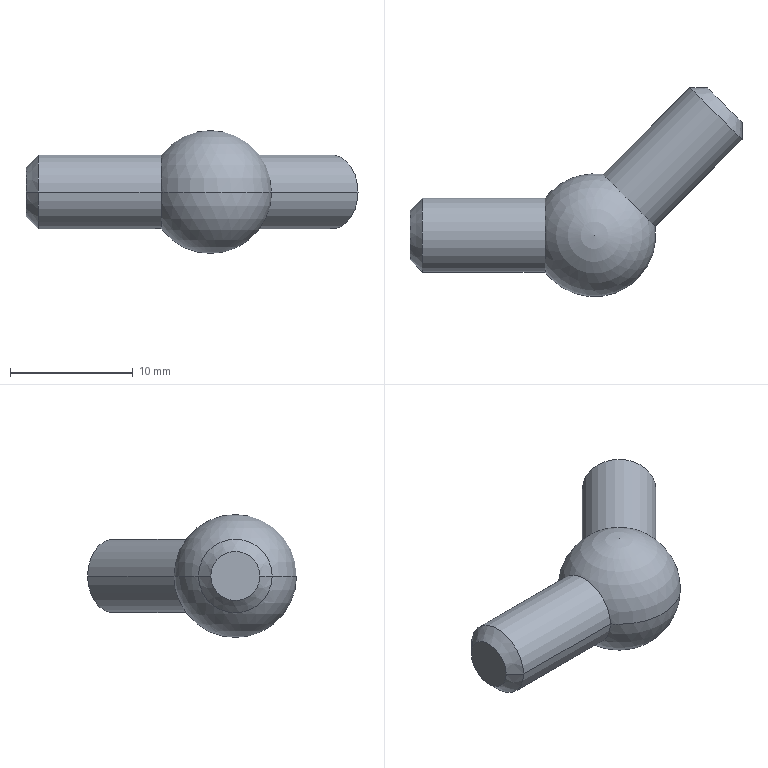Part | STEP file | [B-M6F] | 1 solid | 12 faces | box 27.021 x 17.021 x 10 mm | volume 1100 mm3 | cone 4 | cylinder 4 | sphere 2 | plane 2 | commonest cylinder face diameters 6 x4
STEP:
#1=CARTESIAN_POINT('',(0.,0.,0.));
#2=DIRECTION('',(0.,0.,1.));
#3=DIRECTION('',(1.,0.,0.));
#4=AXIS2_PLACEMENT_3D('',#1,#2,#3);
#5=CARTESIAN_POINT('',(174.099,-132.886,5.));
#6=VERTEX_POINT('',#5);
#7=CARTESIAN_POINT('',(171.271,-130.057,5.));
#8=VERTEX_POINT('',#7);
#9=CARTESIAN_POINT('',(172.685,-131.472,5.));
#10=DIRECTION('',(0.7071,0.7071,0.));
#11=DIRECTION('',(0.7071,-0.7071,0.));
#12=AXIS2_PLACEMENT_3D('',#9,#10,#11);
#13=CIRCLE('',#12,2.);
#14=CARTESIAN_POINT('',(171.978,-132.179,5.));
#15=DIRECTION('',(-0.7071,-0.7071,0.));
#16=DIRECTION('',(-0.7071,0.7071,0.));
#17=AXIS2_PLACEMENT_3D('',#14,#15,#16);
#18=CONICAL_SURFACE('',#17,3.,0.7854);
#19=CARTESIAN_POINT('',(3.142,-1.));
#20=DIRECTION('',(-1.,0.));
#21=VECTOR('',#20,1.);
#22=LINE('',#19,#21);
#23=(GEOMETRIC_REPRESENTATION_CONTEXT(2)PARAMETRIC_REPRESENTATION_CONTEXT()REPRESENTATION_CONTEXT('',''));
#24=DEFINITIONAL_REPRESENTATION('',(#22),#23);
#25=PCURVE('',#18,#24);
#26=CARTESIAN_POINT('',(172.685,-131.472,5.));
#27=DIRECTION('',(0.7071,0.7071,0.));
#28=DIRECTION('',(0.7071,-0.7071,0.));
#29=AXIS2_PLACEMENT_3D('',#26,#27,#28);
#30=PLANE('',#29);
#31=CARTESIAN_POINT('',(0.,0.));
#32=DIRECTION('',(1.,0.));
#33=AXIS2_PLACEMENT_2D('',#31,#32);
#34=CIRCLE('',#33,2.);
#35=(GEOMETRIC_REPRESENTATION_CONTEXT(2)PARAMETRIC_REPRESENTATION_CONTEXT()REPRESENTATION_CONTEXT('',''));
#36=DEFINITIONAL_REPRESENTATION('',(#34),#35);
#37=PCURVE('',#30,#36);
#38=SURFACE_CURVE('',#13,(#25,#37),.PCURVE_S1.);
#39=EDGE_CURVE('',#6,#8,#38,.T.);
#40=ORIENTED_EDGE('',*,*,#39,.F.);
#41=CARTESIAN_POINT('',(174.099,-134.3,5.));
#42=VERTEX_POINT('',#41);
#43=CARTESIAN_POINT('',(174.099,-134.3,5.));
#44=DIRECTION('',(0.,-1.,0.));
#45=VECTOR('',#44,1.);
#46=LINE('',#43,#45);
#47=CARTESIAN_POINT('',(3.142,0.));
#48=DIRECTION('',(0.,1.));
#49=VECTOR('',#48,1.);
#50=LINE('',#47,#49);
#51=(GEOMETRIC_REPRESENTATION_CONTEXT(2)PARAMETRIC_REPRESENTATION_CONTEXT()REPRESENTATION_CONTEXT('',''));
#52=DEFINITIONAL_REPRESENTATION('',(#50),#51);
#53=PCURVE('',#18,#52);
#54=CARTESIAN_POINT('',(171.978,-132.179,5.));
#55=DIRECTION('',(-0.7071,-0.7071,0.));
#56=DIRECTION('',(-0.7071,0.7071,0.));
#57=AXIS2_PLACEMENT_3D('',#54,#55,#56);
#58=CONICAL_SURFACE('',#57,3.,0.7854);
#59=CARTESIAN_POINT('',(3.142,0.));
#60=DIRECTION('',(0.,1.));
#61=VECTOR('',#60,1.);
#62=LINE('',#59,#61);
#63=(GEOMETRIC_REPRESENTATION_CONTEXT(2)PARAMETRIC_REPRESENTATION_CONTEXT()REPRESENTATION_CONTEXT('',''));
#64=DEFINITIONAL_REPRESENTATION('',(#62),#63);
#65=PCURVE('',#58,#64);
#66=SURFACE_CURVE('',#46,(#53,#65),.PCURVE_S1.);
#67=EDGE_CURVE('',#6,#42,#66,.T.);
#68=ORIENTED_EDGE('',*,*,#67,.T.);
#69=CARTESIAN_POINT('',(169.856,-130.057,5.));
#70=VERTEX_POINT('',#69);
#71=CARTESIAN_POINT('',(171.978,-132.179,5.));
#72=DIRECTION('',(-0.7071,-0.7071,0.));
#73=DIRECTION('',(0.7071,-0.7071,0.));
#74=AXIS2_PLACEMENT_3D('',#71,#72,#73);
#75=CIRCLE('',#74,3.);
#76=CARTESIAN_POINT('',(-3.142,0.));
#77=DIRECTION('',(1.,0.));
#78=VECTOR('',#77,1.);
#79=LINE('',#76,#78);
#80=(GEOMETRIC_REPRESENTATION_CONTEXT(2)PARAMETRIC_REPRESENTATION_CONTEXT()REPRESENTATION_CONTEXT('',''));
#81=DEFINITIONAL_REPRESENTATION('',(#79),#80);
#82=PCURVE('',#18,#81);
#83=CARTESIAN_POINT('',(172.685,-131.472,5.));
#84=DIRECTION('',(-0.7071,-0.7071,0.));
#85=DIRECTION('',(-0.7071,0.7071,0.));
#86=AXIS2_PLACEMENT_3D('',#83,#84,#85);
#87=CYLINDRICAL_SURFACE('',#86,3.);
#88=CARTESIAN_POINT('',(-3.142,1.));
#89=DIRECTION('',(1.,0.));
#90=VECTOR('',#89,1.);
#91=LINE('',#88,#90);
#92=(GEOMETRIC_REPRESENTATION_CONTEXT(2)PARAMETRIC_REPRESENTATION_CONTEXT()REPRESENTATION_CONTEXT('',''));
#93=DEFINITIONAL_REPRESENTATION('',(#91),#92);
#94=PCURVE('',#87,#93);
#95=SURFACE_CURVE('',#75,(#82,#94),.PCURVE_S1.);
#96=EDGE_CURVE('',#70,#42,#95,.T.);
#97=ORIENTED_EDGE('',*,*,#96,.F.);
#98=CARTESIAN_POINT('',(169.856,-130.057,5.));
#99=DIRECTION('',(-1.,0.,0.));
#100=VECTOR('',#99,1.);
#101=LINE('',#98,#100);
#102=CARTESIAN_POINT('',(0.,0.));
#103=DIRECTION('',(0.,1.));
#104=VECTOR('',#103,1.);
#105=LINE('',#102,#104);
#106=(GEOMETRIC_REPRESENTATION_CONTEXT(2)PARAMETRIC_REPRESENTATION_CONTEXT()REPRESENTATION_CONTEXT('',''));
#107=DEFINITIONAL_REPRESENTATION('',(#105),#106);
#108=PCURVE('',#18,#107);
#109=CARTESIAN_POINT('',(6.283,0.));
#110=DIRECTION('',(0.,1.));
#111=VECTOR('',#110,1.);
#112=LINE('',#109,#111);
#113=(GEOMETRIC_REPRESENTATION_CONTEXT(2)PARAMETRIC_REPRESENTATION_CONTEXT()REPRESENTATION_CONTEXT('',''));
#114=DEFINITIONAL_REPRESENTATION('',(#112),#113);
#115=PCURVE('',#58,#114);
#116=SURFACE_CURVE('',#101,(#108,#115),.PCURVE_S1.);
#117=EDGE_CURVE('',#8,#70,#116,.T.);
#118=ORIENTED_EDGE('',*,*,#117,.F.);
#119=EDGE_LOOP('',(#40,#68,#97,#118));
#120=FACE_BOUND('',#119,.T.);
#121=ADVANCED_FACE('',(#120),#18,.T.);
#122=CARTESIAN_POINT('',(147.078,-140.078,5.));
#123=VERTEX_POINT('',#122);
#124=CARTESIAN_POINT('',(147.078,-144.078,5.));
#125=VERTEX_POINT('',#124);
#126=CARTESIAN_POINT('',(147.078,-142.078,5.));
#127=DIRECTION('',(-1.,0.,0.));
#128=DIRECTION('',(0.,1.,0.));
#129=AXIS2_PLACEMENT_3D('',#126,#127,#128);
#130=CIRCLE('',#129,2.);
#131=CARTESIAN_POINT('',(148.078,-142.078,5.));
#132=DIRECTION('',(1.,0.,0.));
#133=DIRECTION('',(0.,-1.,0.));
#134=AXIS2_PLACEMENT_3D('',#131,#132,#133);
#135=CONICAL_SURFACE('',#134,3.,0.7854);
#136=CARTESIAN_POINT('',(3.142,-1.));
#137=DIRECTION('',(-1.,0.));
#138=VECTOR('',#137,1.);
#139=LINE('',#136,#138);
#140=(GEOMETRIC_REPRESENTATION_CONTEXT(2)PARAMETRIC_REPRESENTATION_CONTEXT()REPRESENTATION_CONTEXT('',''));
#141=DEFINITIONAL_REPRESENTATION('',(#139),#140);
#142=PCURVE('',#135,#141);
#143=CARTESIAN_POINT('',(147.078,-142.078,5.));
#144=DIRECTION('',(-1.,0.,0.));
#145=DIRECTION('',(0.,1.,0.));
#146=AXIS2_PLACEMENT_3D('',#143,#144,#145);
#147=PLANE('',#146);
#148=CARTESIAN_POINT('',(0.,0.));
#149=DIRECTION('',(1.,0.));
#150=AXIS2_PLACEMENT_2D('',#148,#149);
#151=CIRCLE('',#150,2.);
#152=(GEOMETRIC_REPRESENTATION_CONTEXT(2)PARAMETRIC_REPRESENTATION_CONTEXT()REPRESENTATION_CONTEXT('',''));
#153=DEFINITIONAL_REPRESENTATION('',(#151),#152);
#154=PCURVE('',#147,#153);
#155=SURFACE_CURVE('',#130,(#142,#154),.PCURVE_S1.);
#156=EDGE_CURVE('',#123,#125,#155,.T.);
#157=ORIENTED_EDGE('',*,*,#156,.F.);
#158=CARTESIAN_POINT('',(148.078,-139.078,5.));
#159=VERTEX_POINT('',#158);
#160=CARTESIAN_POINT('',(148.078,-139.078,5.));
#161=DIRECTION('',(0.7071,0.7071,0.));
#162=VECTOR('',#161,1.);
#163=LINE('',#160,#162);
#164=CARTESIAN_POINT('',(3.142,0.));
#165=DIRECTION('',(0.,1.));
#166=VECTOR('',#165,1.);
#167=LINE('',#164,#166);
#168=(GEOMETRIC_REPRESENTATION_CONTEXT(2)PARAMETRIC_REPRESENTATION_CONTEXT()REPRESENTATION_CONTEXT('',''));
#169=DEFINITIONAL_REPRESENTATION('',(#167),#168);
#170=PCURVE('',#135,#169);
#171=CARTESIAN_POINT('',(148.078,-142.078,5.));
#172=DIRECTION('',(1.,0.,0.));
#173=DIRECTION('',(0.,-1.,0.));
#174=AXIS2_PLACEMENT_3D('',#171,#172,#173);
#175=CONICAL_SURFACE('',#174,3.,0.7854);
#176=CARTESIAN_POINT('',(3.142,0.));
#177=DIRECTION('',(0.,1.));
#178=VECTOR('',#177,1.);
#179=LINE('',#176,#178);
#180=(GEOMETRIC_REPRESENTATION_CONTEXT(2)PARAMETRIC_REPRESENTATION_CONTEXT()REPRESENTATION_CONTEXT('',''));
#181=DEFINITIONAL_REPRESENTATION('',(#179),#180);
#182=PCURVE('',#175,#181);
#183=SURFACE_CURVE('',#163,(#170,#182),.PCURVE_S1.);
#184=EDGE_CURVE('',#123,#159,#183,.T.);
#185=ORIENTED_EDGE('',*,*,#184,.T.);
#186=CARTESIAN_POINT('',(148.078,-145.078,5.));
#187=VERTEX_POINT('',#186);
#188=CARTESIAN_POINT('',(148.078,-142.078,5.));
#189=DIRECTION('',(1.,0.,0.));
#190=DIRECTION('',(0.,1.,0.));
#191=AXIS2_PLACEMENT_3D('',#188,#189,#190);
#192=CIRCLE('',#191,3.);
#193=CARTESIAN_POINT('',(-3.142,0.));
#194=DIRECTION('',(1.,0.));
#195=VECTOR('',#194,1.);
#196=LINE('',#193,#195);
#197=(GEOMETRIC_REPRESENTATION_CONTEXT(2)PARAMETRIC_REPRESENTATION_CONTEXT()REPRESENTATION_CONTEXT('',''));
#198=DEFINITIONAL_REPRESENTATION('',(#196),#197);
#199=PCURVE('',#135,#198);
#200=CARTESIAN_POINT('',(147.078,-142.078,5.));
#201=DIRECTION('',(1.,0.,0.));
#202=DIRECTION('',(0.,-1.,0.));
#203=AXIS2_PLACEMENT_3D('',#200,#201,#202);
#204=CYLINDRICAL_SURFACE('',#203,3.);
#205=CARTESIAN_POINT('',(-3.142,1.));
#206=DIRECTION('',(1.,0.));
#207=VECTOR('',#206,1.);
#208=LINE('',#205,#207);
#209=(GEOMETRIC_REPRESENTATION_CONTEXT(2)PARAMETRIC_REPRESENTATION_CONTEXT()REPRESENTATION_CONTEXT('',''));
#210=DEFINITIONAL_REPRESENTATION('',(#208),#209);
#211=PCURVE('',#204,#210);
#212=SURFACE_CURVE('',#192,(#199,#211),.PCURVE_S1.);
#213=EDGE_CURVE('',#187,#159,#212,.T.);
#214=ORIENTED_EDGE('',*,*,#213,.F.);
#215=CARTESIAN_POINT('',(148.078,-145.078,5.));
#216=DIRECTION('',(0.7071,-0.7071,0.));
#217=VECTOR('',#216,1.);
#218=LINE('',#215,#217);
#219=CARTESIAN_POINT('',(0.,0.));
#220=DIRECTION('',(0.,1.));
#221=VECTOR('',#220,1.);
#222=LINE('',#219,#221);
#223=(GEOMETRIC_REPRESENTATION_CONTEXT(2)PARAMETRIC_REPRESENTATION_CONTEXT()REPRESENTATION_CONTEXT('',''));
#224=DEFINITIONAL_REPRESENTATION('',(#222),#223);
#225=PCURVE('',#135,#224);
#226=CARTESIAN_POINT('',(6.283,0.));
#227=DIRECTION('',(0.,1.));
#228=VECTOR('',#227,1.);
#229=LINE('',#226,#228);
#230=(GEOMETRIC_REPRESENTATION_CONTEXT(2)PARAMETRIC_REPRESENTATION_CONTEXT()REPRESENTATION_CONTEXT('',''));
#231=DEFINITIONAL_REPRESENTATION('',(#229),#230);
#232=PCURVE('',#175,#231);
#233=SURFACE_CURVE('',#218,(#225,#232),.PCURVE_S1.);
#234=EDGE_CURVE('',#125,#187,#233,.T.);
#235=ORIENTED_EDGE('',*,*,#234,.F.);
#236=EDGE_LOOP('',(#157,#185,#214,#235));
#237=FACE_BOUND('',#236,.T.);
#238=ADVANCED_FACE('',(#237),#135,.T.);
#239=ORIENTED_EDGE('',*,*,#96,.T.);
#240=CARTESIAN_POINT('',(167.028,-141.371,5.));
#241=VERTEX_POINT('',#240);
#242=CARTESIAN_POINT('',(174.806,-133.593,5.));
#243=DIRECTION('',(-0.7071,-0.7071,0.));
#244=VECTOR('',#243,1.);
#245=LINE('',#242,#244);
#246=CARTESIAN_POINT('',(3.142,0.));
#247=DIRECTION('',(0.,1.));
#248=VECTOR('',#247,1.);
#249=LINE('',#246,#248);
#250=(GEOMETRIC_REPRESENTATION_CONTEXT(2)PARAMETRIC_REPRESENTATION_CONTEXT()REPRESENTATION_CONTEXT('',''));
#251=DEFINITIONAL_REPRESENTATION('',(#249),#250);
#252=PCURVE('',#87,#251);
#253=CARTESIAN_POINT('',(172.685,-131.472,5.));
#254=DIRECTION('',(-0.7071,-0.7071,0.));
#255=DIRECTION('',(-0.7071,0.7071,0.));
#256=AXIS2_PLACEMENT_3D('',#253,#254,#255);
#257=CYLINDRICAL_SURFACE('',#256,3.);
#258=CARTESIAN_POINT('',(3.142,0.));
#259=DIRECTION('',(0.,1.));
#260=VECTOR('',#259,1.);
#261=LINE('',#258,#260);
#262=(GEOMETRIC_REPRESENTATION_CONTEXT(2)PARAMETRIC_REPRESENTATION_CONTEXT()REPRESENTATION_CONTEXT('',''));
#263=DEFINITIONAL_REPRESENTATION('',(#261),#262);
#264=PCURVE('',#257,#263);
#265=SURFACE_CURVE('',#245,(#252,#264),.PCURVE_S1.);
#266=EDGE_CURVE('',#42,#241,#265,.T.);
#267=ORIENTED_EDGE('',*,*,#266,.T.);
#268=CARTESIAN_POINT('',(162.785,-137.128,5.));
#269=VERTEX_POINT('',#268);
#270=CARTESIAN_POINT('',(164.907,-139.25,5.));
#271=DIRECTION('',(0.7071,0.7071,0.));
#272=DIRECTION('',(-0.7071,0.7071,0.));
#273=AXIS2_PLACEMENT_3D('',#270,#271,#272);
#274=CIRCLE('',#273,3.);
#275=CARTESIAN_POINT('',(6.283,11.));
#276=DIRECTION('',(-1.,0.));
#277=VECTOR('',#276,1.);
#278=LINE('',#275,#277);
#279=(GEOMETRIC_REPRESENTATION_CONTEXT(2)PARAMETRIC_REPRESENTATION_CONTEXT()REPRESENTATION_CONTEXT('',''));
#280=DEFINITIONAL_REPRESENTATION('',(#278),#279);
#281=PCURVE('',#87,#280);
#282=CARTESIAN_POINT('',(162.078,-142.078,5.));
#283=DIRECTION('',(0.,0.,-1.));
#284=DIRECTION('',(-0.7071,0.7071,0.));
#285=AXIS2_PLACEMENT_3D('',#282,#283,#284);
#286=SPHERICAL_SURFACE('',#285,5.);
#287=CARTESIAN_POINT('',(2.214,0.));
#288=CARTESIAN_POINT('',(2.214,0.02855));
#289=CARTESIAN_POINT('',(2.211,0.08568));
#290=CARTESIAN_POINT('',(2.196,0.1702));
#291=CARTESIAN_POINT('',(2.171,0.2525));
#292=CARTESIAN_POINT('',(2.136,0.3312));
#293=CARTESIAN_POINT('',(2.088,0.4049));
#294=CARTESIAN_POINT('',(2.029,0.472));
#295=CARTESIAN_POINT('',(1.958,0.5308));
#296=CARTESIAN_POINT('',(1.875,0.5793));
#297=CARTESIAN_POINT('',(1.78,0.6158));
#298=CARTESIAN_POINT('',(1.678,0.6384));
#299=CARTESIAN_POINT('',(1.571,0.6461));
#300=CARTESIAN_POINT('',(1.464,0.6384));
#301=CARTESIAN_POINT('',(1.361,0.6158));
#302=CARTESIAN_POINT('',(1.267,0.5793));
#303=CARTESIAN_POINT('',(1.184,0.5308));
#304=CARTESIAN_POINT('',(1.112,0.472));
#305=CARTESIAN_POINT('',(1.053,0.4049));
#306=CARTESIAN_POINT('',(1.006,0.3312));
#307=CARTESIAN_POINT('',(0.9703,0.2525));
#308=CARTESIAN_POINT('',(0.9453,0.1702));
#309=CARTESIAN_POINT('',(0.9305,0.08568));
#310=CARTESIAN_POINT('',(0.9273,0.02855));
#311=CARTESIAN_POINT('',(0.9273,0.));
#312=B_SPLINE_CURVE_WITH_KNOTS('',3,(#287,#288,#289,#290,#291,#292,#293,#294,#295,#296,#297,#298,#299,#300,#301,#302,#303,#304,#305,#306,#307,#308,#309,#310,#311),.UNSPECIFIED.,.F.,.F.,(4,1,1,1,1,1,1,1,1,1,1,1,1,1,1,1,1,1,1,1,1,1,4),(3.142,3.284,3.427,3.57,3.713,3.856,3.998,4.141,4.284,4.427,4.57,4.712,4.855,4.998,5.141,5.284,5.426,5.569,5.712,5.855,5.998,6.14,6.283),.QUASI_UNIFORM_KNOTS.);
#313=(GEOMETRIC_REPRESENTATION_CONTEXT(2)PARAMETRIC_REPRESENTATION_CONTEXT()REPRESENTATION_CONTEXT('',''));
#314=DEFINITIONAL_REPRESENTATION('',(#312),#313);
#315=PCURVE('',#286,#314);
#316=SURFACE_CURVE('',#274,(#281,#315),.PCURVE_S1.);
#317=EDGE_CURVE('',#241,#269,#316,.T.);
#318=ORIENTED_EDGE('',*,*,#317,.T.);
#319=CARTESIAN_POINT('',(170.563,-129.35,5.));
#320=DIRECTION('',(-0.7071,-0.7071,0.));
#321=VECTOR('',#320,1.);
#322=LINE('',#319,#321);
#323=CARTESIAN_POINT('',(0.,0.));
#324=DIRECTION('',(0.,1.));
#325=VECTOR('',#324,1.);
#326=LINE('',#323,#325);
#327=(GEOMETRIC_REPRESENTATION_CONTEXT(2)PARAMETRIC_REPRESENTATION_CONTEXT()REPRESENTATION_CONTEXT('',''));
#328=DEFINITIONAL_REPRESENTATION('',(#326),#327);
#329=PCURVE('',#87,#328);
#330=CARTESIAN_POINT('',(6.283,0.));
#331=DIRECTION('',(0.,1.));
#332=VECTOR('',#331,1.);
#333=LINE('',#330,#332);
#334=(GEOMETRIC_REPRESENTATION_CONTEXT(2)PARAMETRIC_REPRESENTATION_CONTEXT()REPRESENTATION_CONTEXT('',''));
#335=DEFINITIONAL_REPRESENTATION('',(#333),#334);
#336=PCURVE('',#257,#335);
#337=SURFACE_CURVE('',#322,(#329,#336),.PCURVE_S1.);
#338=EDGE_CURVE('',#70,#269,#337,.T.);
#339=ORIENTED_EDGE('',*,*,#338,.F.);
#340=EDGE_LOOP('',(#239,#267,#318,#339));
#341=FACE_BOUND('',#340,.T.);
#342=ADVANCED_FACE('',(#341),#87,.T.);
#343=ORIENTED_EDGE('',*,*,#317,.F.);
#344=CARTESIAN_POINT('',(158.543,-145.614,5.));
#345=VERTEX_POINT('',#344);
#346=CARTESIAN_POINT('',(162.078,-142.078,5.));
#347=DIRECTION('',(0.,0.,-1.));
#348=DIRECTION('',(-1.,0.,0.));
#349=AXIS2_PLACEMENT_3D('',#346,#347,#348);
#350=CIRCLE('',#349,5.);
#351=CARTESIAN_POINT('',(-0.7854,0.));
#352=DIRECTION('',(1.,0.));
#353=VECTOR('',#352,1.);
#354=LINE('',#351,#353);
#355=(GEOMETRIC_REPRESENTATION_CONTEXT(2)PARAMETRIC_REPRESENTATION_CONTEXT()REPRESENTATION_CONTEXT('',''));
#356=DEFINITIONAL_REPRESENTATION('',(#354),#355);
#357=PCURVE('',#286,#356);
#358=CARTESIAN_POINT('',(162.078,-142.078,5.));
#359=DIRECTION('',(0.,0.,-1.));
#360=DIRECTION('',(-0.7071,0.7071,0.));
#361=AXIS2_PLACEMENT_3D('',#358,#359,#360);
#362=SPHERICAL_SURFACE('',#361,5.);
#363=CARTESIAN_POINT('',(-0.7854,0.));
#364=DIRECTION('',(1.,0.));
#365=VECTOR('',#364,1.);
#366=LINE('',#363,#365);
#367=(GEOMETRIC_REPRESENTATION_CONTEXT(2)PARAMETRIC_REPRESENTATION_CONTEXT()REPRESENTATION_CONTEXT('',''));
#368=DEFINITIONAL_REPRESENTATION('',(#366),#367);
#369=PCURVE('',#362,#368);
#370=SURFACE_CURVE('',#350,(#357,#369),.PCURVE_S1.);
#371=EDGE_CURVE('',#241,#345,#370,.T.);
#372=ORIENTED_EDGE('',*,*,#371,.T.);
#373=CARTESIAN_POINT('',(158.078,-145.078,5.));
#374=VERTEX_POINT('',#373);
#375=CARTESIAN_POINT('',(162.078,-142.078,5.));
#376=DIRECTION('',(0.,0.,1.));
#377=DIRECTION('',(1.,0.,0.));
#378=AXIS2_PLACEMENT_3D('',#375,#376,#377);
#379=CIRCLE('',#378,5.);
#380=CARTESIAN_POINT('',(8.639,0.));
#381=DIRECTION('',(-1.,0.));
#382=VECTOR('',#381,1.);
#383=LINE('',#380,#382);
#384=(GEOMETRIC_REPRESENTATION_CONTEXT(2)PARAMETRIC_REPRESENTATION_CONTEXT()REPRESENTATION_CONTEXT('',''));
#385=DEFINITIONAL_REPRESENTATION('',(#383),#384);
#386=PCURVE('',#286,#385);
#387=CARTESIAN_POINT('',(8.639,0.));
#388=DIRECTION('',(-1.,0.));
#389=VECTOR('',#388,1.);
#390=LINE('',#387,#389);
#391=(GEOMETRIC_REPRESENTATION_CONTEXT(2)PARAMETRIC_REPRESENTATION_CONTEXT()REPRESENTATION_CONTEXT('',''));
#392=DEFINITIONAL_REPRESENTATION('',(#390),#391);
#393=PCURVE('',#362,#392);
#394=SURFACE_CURVE('',#379,(#386,#393),.PCURVE_S1.);
#395=EDGE_CURVE('',#374,#345,#394,.T.);
#396=ORIENTED_EDGE('',*,*,#395,.F.);
#397=CARTESIAN_POINT('',(158.078,-139.078,5.));
#398=VERTEX_POINT('',#397);
#399=CARTESIAN_POINT('',(158.078,-142.078,5.));
#400=DIRECTION('',(-1.,0.,0.));
#401=DIRECTION('',(0.,-1.,0.));
#402=AXIS2_PLACEMENT_3D('',#399,#400,#401);
#403=CIRCLE('',#402,3.);
#404=CARTESIAN_POINT('',(6.141,0.));
#405=CARTESIAN_POINT('',(6.141,0.02855));
#406=CARTESIAN_POINT('',(6.138,0.08568));
#407=CARTESIAN_POINT('',(6.123,0.1702));
#408=CARTESIAN_POINT('',(6.098,0.2525));
#409=CARTESIAN_POINT('',(6.063,0.3312));
#410=CARTESIAN_POINT('',(6.015,0.4049));
#411=CARTESIAN_POINT('',(5.956,0.472));
#412=CARTESIAN_POINT('',(5.885,0.5308));
#413=CARTESIAN_POINT('',(5.802,0.5793));
#414=CARTESIAN_POINT('',(5.707,0.6158));
#415=CARTESIAN_POINT('',(5.605,0.6384));
#416=CARTESIAN_POINT('',(5.498,0.6461));
#417=CARTESIAN_POINT('',(5.391,0.6384));
#418=CARTESIAN_POINT('',(5.288,0.6158));
#419=CARTESIAN_POINT('',(5.194,0.5793));
#420=CARTESIAN_POINT('',(5.111,0.5308));
#421=CARTESIAN_POINT('',(5.039,0.472));
#422=CARTESIAN_POINT('',(4.98,0.4049));
#423=CARTESIAN_POINT('',(4.933,0.3312));
#424=CARTESIAN_POINT('',(4.897,0.2525));
#425=CARTESIAN_POINT('',(4.872,0.1702));
#426=CARTESIAN_POINT('',(4.858,0.08568));
#427=CARTESIAN_POINT('',(4.854,0.02855));
#428=CARTESIAN_POINT('',(4.854,0.));
#429=B_SPLINE_CURVE_WITH_KNOTS('',3,(#404,#405,#406,#407,#408,#409,#410,#411,#412,#413,#414,#415,#416,#417,#418,#419,#420,#421,#422,#423,#424,#425,#426,#427,#428),.UNSPECIFIED.,.F.,.F.,(4,1,1,1,1,1,1,1,1,1,1,1,1,1,1,1,1,1,1,1,1,1,4),(3.142,3.284,3.427,3.57,3.713,3.856,3.998,4.141,4.284,4.427,4.57,4.712,4.855,4.998,5.141,5.284,5.426,5.569,5.712,5.855,5.998,6.14,6.283),.QUASI_UNIFORM_KNOTS.);
#430=(GEOMETRIC_REPRESENTATION_CONTEXT(2)PARAMETRIC_REPRESENTATION_CONTEXT()REPRESENTATION_CONTEXT('',''));
#431=DEFINITIONAL_REPRESENTATION('',(#429),#430);
#432=PCURVE('',#286,#431);
#433=CARTESIAN_POINT('',(6.283,11.));
#434=DIRECTION('',(-1.,0.));
#435=VECTOR('',#434,1.);
#436=LINE('',#433,#435);
#437=(GEOMETRIC_REPRESENTATION_CONTEXT(2)PARAMETRIC_REPRESENTATION_CONTEXT()REPRESENTATION_CONTEXT('',''));
#438=DEFINITIONAL_REPRESENTATION('',(#436),#437);
#439=PCURVE('',#204,#438);
#440=SURFACE_CURVE('',#403,(#432,#439),.PCURVE_S1.);
#441=EDGE_CURVE('',#398,#374,#440,.T.);
#442=ORIENTED_EDGE('',*,*,#441,.F.);
#443=CARTESIAN_POINT('',(158.543,-138.543,5.));
#444=VERTEX_POINT('',#443);
#445=CARTESIAN_POINT('',(162.078,-142.078,5.));
#446=DIRECTION('',(0.,0.,1.));
#447=DIRECTION('',(1.,0.,0.));
#448=AXIS2_PLACEMENT_3D('',#445,#446,#447);
#449=CIRCLE('',#448,5.);
#450=CARTESIAN_POINT('',(7.21,0.));
#451=CARTESIAN_POINT('',(7.194,0.));
#452=CARTESIAN_POINT('',(7.162,0.));
#453=CARTESIAN_POINT('',(7.113,0.));
#454=CARTESIAN_POINT('',(7.065,0.));
#455=CARTESIAN_POINT('',(7.016,0.));
#456=CARTESIAN_POINT('',(6.967,0.));
#457=CARTESIAN_POINT('',(6.919,0.));
#458=CARTESIAN_POINT('',(6.87,0.));
#459=CARTESIAN_POINT('',(6.822,0.));
#460=CARTESIAN_POINT('',(6.773,0.));
#461=CARTESIAN_POINT('',(6.724,0.));
#462=CARTESIAN_POINT('',(6.676,0.));
#463=CARTESIAN_POINT('',(6.627,0.));
#464=CARTESIAN_POINT('',(6.579,0.));
#465=CARTESIAN_POINT('',(6.53,0.));
#466=CARTESIAN_POINT('',(6.481,0.));
#467=CARTESIAN_POINT('',(6.433,0.));
#468=CARTESIAN_POINT('',(6.384,0.));
#469=CARTESIAN_POINT('',(6.336,0.));
#470=CARTESIAN_POINT('',(6.287,0.));
#471=CARTESIAN_POINT('',(6.238,0.));
#472=CARTESIAN_POINT('',(6.19,0.));
#473=CARTESIAN_POINT('',(6.157,0.));
#474=CARTESIAN_POINT('',(6.141,0.));
#475=B_SPLINE_CURVE_WITH_KNOTS('',3,(#450,#451,#452,#453,#454,#455,#456,#457,#458,#459,#460,#461,#462,#463,#464,#465,#466,#467,#468,#469,#470,#471,#472,#473,#474),.UNSPECIFIED.,.F.,.F.,(4,1,1,1,1,1,1,1,1,1,1,1,1,1,1,1,1,1,1,1,1,1,4),(1.429,1.477,1.526,1.575,1.623,1.672,1.72,1.769,1.818,1.866,1.915,1.963,2.012,2.061,2.109,2.158,2.206,2.255,2.304,2.352,2.401,2.449,2.498),.QUASI_UNIFORM_KNOTS.);
#476=(GEOMETRIC_REPRESENTATION_CONTEXT(2)PARAMETRIC_REPRESENTATION_CONTEXT()REPRESENTATION_CONTEXT('',''));
#477=DEFINITIONAL_REPRESENTATION('',(#475),#476);
#478=PCURVE('',#286,#477);
#479=CARTESIAN_POINT('',(6.283,0.));
#480=CARTESIAN_POINT('',(6.281,0.));
#481=CARTESIAN_POINT('',(6.277,0.));
#482=CARTESIAN_POINT('',(6.27,0.));
#483=CARTESIAN_POINT('',(6.264,0.));
#484=CARTESIAN_POINT('',(6.257,0.));
#485=CARTESIAN_POINT('',(6.251,0.));
#486=CARTESIAN_POINT('',(6.244,0.));
#487=CARTESIAN_POINT('',(6.238,0.));
#488=CARTESIAN_POINT('',(6.232,0.));
#489=CARTESIAN_POINT('',(6.225,0.));
#490=CARTESIAN_POINT('',(6.219,0.));
#491=CARTESIAN_POINT('',(6.212,0.));
#492=CARTESIAN_POINT('',(6.206,0.));
#493=CARTESIAN_POINT('',(6.199,0.));
#494=CARTESIAN_POINT('',(6.193,0.));
#495=CARTESIAN_POINT('',(6.186,0.));
#496=CARTESIAN_POINT('',(6.18,0.));
#497=CARTESIAN_POINT('',(6.174,0.));
#498=CARTESIAN_POINT('',(6.167,0.));
#499=CARTESIAN_POINT('',(6.161,0.));
#500=CARTESIAN_POINT('',(6.154,0.));
#501=CARTESIAN_POINT('',(6.148,0.));
#502=CARTESIAN_POINT('',(6.143,0.));
#503=CARTESIAN_POINT('',(6.141,0.));
#504=B_SPLINE_CURVE_WITH_KNOTS('',3,(#479,#480,#481,#482,#483,#484,#485,#486,#487,#488,#489,#490,#491,#492,#493,#494,#495,#496,#497,#498,#499,#500,#501,#502,#503),.UNSPECIFIED.,.F.,.F.,(4,1,1,1,1,1,1,1,1,1,1,1,1,1,1,1,1,1,1,1,1,1,4),(2.356,2.363,2.369,2.376,2.382,2.388,2.395,2.401,2.408,2.414,2.421,2.427,2.434,2.44,2.446,2.453,2.459,2.466,2.472,2.479,2.485,2.492,2.498),.QUASI_UNIFORM_KNOTS.);
#505=(GEOMETRIC_REPRESENTATION_CONTEXT(2)PARAMETRIC_REPRESENTATION_CONTEXT()REPRESENTATION_CONTEXT('',''));
#506=DEFINITIONAL_REPRESENTATION('',(#504),#505);
#507=PCURVE('',#362,#506);
#508=SURFACE_CURVE('',#449,(#478,#507),.PCURVE_S1.);
#509=EDGE_CURVE('',#444,#398,#508,.T.);
#510=ORIENTED_EDGE('',*,*,#509,.F.);
#511=CARTESIAN_POINT('',(162.078,-142.078,0.));
#512=VERTEX_POINT('',#511);
#513=CARTESIAN_POINT('',(158.543,-138.543,5.));
#514=CARTESIAN_POINT('',(158.543,-138.543,3.691));
#515=CARTESIAN_POINT('',(158.833,-138.833,2.382));
#516=CARTESIAN_POINT('',(159.415,-139.415,1.234));
#517=CARTESIAN_POINT('',(160.227,-140.227,0.4111));
#518=CARTESIAN_POINT('',(161.153,-141.153,0.));
#519=CARTESIAN_POINT('',(162.078,-142.078,0.));
#520=B_SPLINE_CURVE_WITH_KNOTS('',6,(#513,#514,#515,#516,#517,#518,#519),.UNSPECIFIED.,.F.,.F.,(7,7),(0.,1.571),.PIECEWISE_BEZIER_KNOTS.);
#521=CARTESIAN_POINT('',(6.283,0.));
#522=DIRECTION('',(0.,1.));
#523=VECTOR('',#522,1.);
#524=LINE('',#521,#523);
#525=(GEOMETRIC_REPRESENTATION_CONTEXT(2)PARAMETRIC_REPRESENTATION_CONTEXT()REPRESENTATION_CONTEXT('',''));
#526=DEFINITIONAL_REPRESENTATION('',(#524),#525);
#527=PCURVE('',#286,#526);
#528=CARTESIAN_POINT('',(0.,0.));
#529=DIRECTION('',(0.,1.));
#530=VECTOR('',#529,1.);
#531=LINE('',#528,#530);
#532=(GEOMETRIC_REPRESENTATION_CONTEXT(2)PARAMETRIC_REPRESENTATION_CONTEXT()REPRESENTATION_CONTEXT('',''));
#533=DEFINITIONAL_REPRESENTATION('',(#531),#532);
#534=PCURVE('',#286,#533);
#535=SEAM_CURVE('',#520,(#527,#534),.PCURVE_S1.);
#536=EDGE_CURVE('',#444,#512,#535,.T.);
#537=ORIENTED_EDGE('',*,*,#536,.T.);
#538=ORIENTED_EDGE('',*,*,#536,.F.);
#539=CARTESIAN_POINT('',(162.078,-142.078,5.));
#540=DIRECTION('',(0.,0.,1.));
#541=DIRECTION('',(1.,0.,0.));
#542=AXIS2_PLACEMENT_3D('',#539,#540,#541);
#543=CIRCLE('',#542,5.);
#544=CARTESIAN_POINT('',(0.9273,0.));
#545=CARTESIAN_POINT('',(0.9111,0.));
#546=CARTESIAN_POINT('',(0.8787,0.));
#547=CARTESIAN_POINT('',(0.8301,0.));
#548=CARTESIAN_POINT('',(0.7815,0.));
#549=CARTESIAN_POINT('',(0.7329,0.));
#550=CARTESIAN_POINT('',(0.6843,0.));
#551=CARTESIAN_POINT('',(0.6357,0.));
#552=CARTESIAN_POINT('',(0.5871,0.));
#553=CARTESIAN_POINT('',(0.5385,0.));
#554=CARTESIAN_POINT('',(0.4899,0.));
#555=CARTESIAN_POINT('',(0.4413,0.));
#556=CARTESIAN_POINT('',(0.3927,0.));
#557=CARTESIAN_POINT('',(0.3441,0.));
#558=CARTESIAN_POINT('',(0.2955,0.));
#559=CARTESIAN_POINT('',(0.2469,0.));
#560=CARTESIAN_POINT('',(0.1983,0.));
#561=CARTESIAN_POINT('',(0.1497,0.));
#562=CARTESIAN_POINT('',(0.1011,0.));
#563=CARTESIAN_POINT('',(0.0525,0.));
#564=CARTESIAN_POINT('',(0.003902,0.));
#565=CARTESIAN_POINT('',(-0.0447,0.));
#566=CARTESIAN_POINT('',(-0.0933,0.));
#567=CARTESIAN_POINT('',(-0.1257,0.));
#568=CARTESIAN_POINT('',(-0.1419,0.));
#569=B_SPLINE_CURVE_WITH_KNOTS('',3,(#544,#545,#546,#547,#548,#549,#550,#551,#552,#553,#554,#555,#556,#557,#558,#559,#560,#561,#562,#563,#564,#565,#566,#567,#568),.UNSPECIFIED.,.F.,.F.,(4,1,1,1,1,1,1,1,1,1,1,1,1,1,1,1,1,1,1,1,1,1,4),(1.429,1.477,1.526,1.575,1.623,1.672,1.72,1.769,1.818,1.866,1.915,1.963,2.012,2.061,2.109,2.158,2.206,2.255,2.304,2.352,2.401,2.449,2.498),.QUASI_UNIFORM_KNOTS.);
#570=(GEOMETRIC_REPRESENTATION_CONTEXT(2)PARAMETRIC_REPRESENTATION_CONTEXT()REPRESENTATION_CONTEXT('',''));
#571=DEFINITIONAL_REPRESENTATION('',(#569),#570);
#572=PCURVE('',#286,#571);
#573=CARTESIAN_POINT('',(2.356,0.));
#574=DIRECTION('',(-1.,0.));
#575=VECTOR('',#574,1.);
#576=LINE('',#573,#575);
#577=(GEOMETRIC_REPRESENTATION_CONTEXT(2)PARAMETRIC_REPRESENTATION_CONTEXT()REPRESENTATION_CONTEXT('',''));
#578=DEFINITIONAL_REPRESENTATION('',(#576),#577);
#579=PCURVE('',#362,#578);
#580=SURFACE_CURVE('',#543,(#572,#579),.PCURVE_S1.);
#581=EDGE_CURVE('',#269,#444,#580,.T.);
#582=ORIENTED_EDGE('',*,*,#581,.F.);
#583=EDGE_LOOP('',(#343,#372,#396,#442,#510,#537,#538,#582));
#584=FACE_BOUND('',#583,.T.);
#585=ADVANCED_FACE('',(#584),#286,.T.);
#586=ORIENTED_EDGE('',*,*,#213,.T.);
#587=CARTESIAN_POINT('',(147.078,-139.078,5.));
#588=DIRECTION('',(1.,0.,0.));
#589=VECTOR('',#588,1.);
#590=LINE('',#587,#589);
#591=CARTESIAN_POINT('',(3.142,0.));
#592=DIRECTION('',(0.,1.));
#593=VECTOR('',#592,1.);
#594=LINE('',#591,#593);
#595=(GEOMETRIC_REPRESENTATION_CONTEXT(2)PARAMETRIC_REPRESENTATION_CONTEXT()REPRESENTATION_CONTEXT('',''));
#596=DEFINITIONAL_REPRESENTATION('',(#594),#595);
#597=PCURVE('',#204,#596);
#598=CARTESIAN_POINT('',(147.078,-142.078,5.));
#599=DIRECTION('',(1.,0.,0.));
#600=DIRECTION('',(0.,-1.,0.));
#601=AXIS2_PLACEMENT_3D('',#598,#599,#600);
#602=CYLINDRICAL_SURFACE('',#601,3.);
#603=CARTESIAN_POINT('',(3.142,0.));
#604=DIRECTION('',(0.,1.));
#605=VECTOR('',#604,1.);
#606=LINE('',#603,#605);
#607=(GEOMETRIC_REPRESENTATION_CONTEXT(2)PARAMETRIC_REPRESENTATION_CONTEXT()REPRESENTATION_CONTEXT('',''));
#608=DEFINITIONAL_REPRESENTATION('',(#606),#607);
#609=PCURVE('',#602,#608);
#610=SURFACE_CURVE('',#590,(#597,#609),.PCURVE_S1.);
#611=EDGE_CURVE('',#159,#398,#610,.T.);
#612=ORIENTED_EDGE('',*,*,#611,.T.);
#613=ORIENTED_EDGE('',*,*,#441,.T.);
#614=CARTESIAN_POINT('',(147.078,-145.078,5.));
#615=DIRECTION('',(1.,0.,0.));
#616=VECTOR('',#615,1.);
#617=LINE('',#614,#616);
#618=CARTESIAN_POINT('',(0.,0.));
#619=DIRECTION('',(0.,1.));
#620=VECTOR('',#619,1.);
#621=LINE('',#618,#620);
#622=(GEOMETRIC_REPRESENTATION_CONTEXT(2)PARAMETRIC_REPRESENTATION_CONTEXT()REPRESENTATION_CONTEXT('',''));
#623=DEFINITIONAL_REPRESENTATION('',(#621),#622);
#624=PCURVE('',#204,#623);
#625=CARTESIAN_POINT('',(6.283,0.));
#626=DIRECTION('',(0.,1.));
#627=VECTOR('',#626,1.);
#628=LINE('',#625,#627);
#629=(GEOMETRIC_REPRESENTATION_CONTEXT(2)PARAMETRIC_REPRESENTATION_CONTEXT()REPRESENTATION_CONTEXT('',''));
#630=DEFINITIONAL_REPRESENTATION('',(#628),#629);
#631=PCURVE('',#602,#630);
#632=SURFACE_CURVE('',#617,(#624,#631),.PCURVE_S1.);
#633=EDGE_CURVE('',#187,#374,#632,.T.);
#634=ORIENTED_EDGE('',*,*,#633,.F.);
#635=EDGE_LOOP('',(#586,#612,#613,#634));
#636=FACE_BOUND('',#635,.T.);
#637=ADVANCED_FACE('',(#636),#204,.T.);
#638=CARTESIAN_POINT('',(147.078,-142.078,5.));
#639=DIRECTION('',(-1.,0.,0.));
#640=DIRECTION('',(0.,1.,0.));
#641=AXIS2_PLACEMENT_3D('',#638,#639,#640);
#642=CIRCLE('',#641,2.);
#643=CARTESIAN_POINT('',(0.,0.));
#644=DIRECTION('',(1.,0.));
#645=AXIS2_PLACEMENT_2D('',#643,#644);
#646=CIRCLE('',#645,2.);
#647=(GEOMETRIC_REPRESENTATION_CONTEXT(2)PARAMETRIC_REPRESENTATION_CONTEXT()REPRESENTATION_CONTEXT('',''));
#648=DEFINITIONAL_REPRESENTATION('',(#646),#647);
#649=PCURVE('',#147,#648);
#650=CARTESIAN_POINT('',(9.425,-1.));
#651=DIRECTION('',(-1.,0.));
#652=VECTOR('',#651,1.);
#653=LINE('',#650,#652);
#654=(GEOMETRIC_REPRESENTATION_CONTEXT(2)PARAMETRIC_REPRESENTATION_CONTEXT()REPRESENTATION_CONTEXT('',''));
#655=DEFINITIONAL_REPRESENTATION('',(#653),#654);
#656=PCURVE('',#175,#655);
#657=SURFACE_CURVE('',#642,(#649,#656),.PCURVE_S1.);
#658=EDGE_CURVE('',#125,#123,#657,.T.);
#659=ORIENTED_EDGE('',*,*,#658,.T.);
#660=ORIENTED_EDGE('',*,*,#156,.T.);
#661=EDGE_LOOP('',(#659,#660));
#662=FACE_BOUND('',#661,.T.);
#663=ADVANCED_FACE('',(#662),#147,.T.);
#664=ORIENTED_EDGE('',*,*,#611,.F.);
#665=CARTESIAN_POINT('',(148.078,-142.078,5.));
#666=DIRECTION('',(1.,0.,0.));
#667=DIRECTION('',(0.,1.,0.));
#668=AXIS2_PLACEMENT_3D('',#665,#666,#667);
#669=CIRCLE('',#668,3.);
#670=CARTESIAN_POINT('',(3.142,1.));
#671=DIRECTION('',(1.,0.));
#672=VECTOR('',#671,1.);
#673=LINE('',#670,#672);
#674=(GEOMETRIC_REPRESENTATION_CONTEXT(2)PARAMETRIC_REPRESENTATION_CONTEXT()REPRESENTATION_CONTEXT('',''));
#675=DEFINITIONAL_REPRESENTATION('',(#673),#674);
#676=PCURVE('',#602,#675);
#677=CARTESIAN_POINT('',(3.142,0.));
#678=DIRECTION('',(1.,0.));
#679=VECTOR('',#678,1.);
#680=LINE('',#677,#679);
#681=(GEOMETRIC_REPRESENTATION_CONTEXT(2)PARAMETRIC_REPRESENTATION_CONTEXT()REPRESENTATION_CONTEXT('',''));
#682=DEFINITIONAL_REPRESENTATION('',(#680),#681);
#683=PCURVE('',#175,#682);
#684=SURFACE_CURVE('',#669,(#676,#683),.PCURVE_S1.);
#685=EDGE_CURVE('',#159,#187,#684,.T.);
#686=ORIENTED_EDGE('',*,*,#685,.T.);
#687=ORIENTED_EDGE('',*,*,#633,.T.);
#688=CARTESIAN_POINT('',(158.078,-142.078,5.));
#689=DIRECTION('',(-1.,0.,0.));
#690=DIRECTION('',(0.,-1.,0.));
#691=AXIS2_PLACEMENT_3D('',#688,#689,#690);
#692=CIRCLE('',#691,3.);
#693=CARTESIAN_POINT('',(6.283,11.));
#694=DIRECTION('',(-1.,0.));
#695=VECTOR('',#694,1.);
#696=LINE('',#693,#695);
#697=(GEOMETRIC_REPRESENTATION_CONTEXT(2)PARAMETRIC_REPRESENTATION_CONTEXT()REPRESENTATION_CONTEXT('',''));
#698=DEFINITIONAL_REPRESENTATION('',(#696),#697);
#699=PCURVE('',#602,#698);
#700=CARTESIAN_POINT('',(4.854,0.));
#701=CARTESIAN_POINT('',(4.854,-0.02855));
#702=CARTESIAN_POINT('',(4.858,-0.08568));
#703=CARTESIAN_POINT('',(4.872,-0.1702));
#704=CARTESIAN_POINT('',(4.897,-0.2525));
#705=CARTESIAN_POINT('',(4.933,-0.3312));
#706=CARTESIAN_POINT('',(4.98,-0.4049));
#707=CARTESIAN_POINT('',(5.039,-0.472));
#708=CARTESIAN_POINT('',(5.111,-0.5308));
#709=CARTESIAN_POINT('',(5.194,-0.5793));
#710=CARTESIAN_POINT('',(5.288,-0.6158));
#711=CARTESIAN_POINT('',(5.391,-0.6384));
#712=CARTESIAN_POINT('',(5.498,-0.6461));
#713=CARTESIAN_POINT('',(5.605,-0.6384));
#714=CARTESIAN_POINT('',(5.707,-0.6158));
#715=CARTESIAN_POINT('',(5.802,-0.5793));
#716=CARTESIAN_POINT('',(5.885,-0.5308));
#717=CARTESIAN_POINT('',(5.956,-0.472));
#718=CARTESIAN_POINT('',(6.015,-0.4049));
#719=CARTESIAN_POINT('',(6.063,-0.3312));
#720=CARTESIAN_POINT('',(6.098,-0.2525));
#721=CARTESIAN_POINT('',(6.123,-0.1702));
#722=CARTESIAN_POINT('',(6.138,-0.08568));
#723=CARTESIAN_POINT('',(6.141,-0.02855));
#724=CARTESIAN_POINT('',(6.141,0.));
#725=B_SPLINE_CURVE_WITH_KNOTS('',3,(#700,#701,#702,#703,#704,#705,#706,#707,#708,#709,#710,#711,#712,#713,#714,#715,#716,#717,#718,#719,#720,#721,#722,#723,#724),.UNSPECIFIED.,.F.,.F.,(4,1,1,1,1,1,1,1,1,1,1,1,1,1,1,1,1,1,1,1,1,1,4),(0.,0.1428,0.2856,0.4284,0.5712,0.714,0.8568,0.9996,1.142,1.285,1.428,1.571,1.714,1.856,1.999,2.142,2.285,2.428,2.57,2.713,2.856,2.999,3.142),.QUASI_UNIFORM_KNOTS.);
#726=(GEOMETRIC_REPRESENTATION_CONTEXT(2)PARAMETRIC_REPRESENTATION_CONTEXT()REPRESENTATION_CONTEXT('',''));
#727=DEFINITIONAL_REPRESENTATION('',(#725),#726);
#728=PCURVE('',#362,#727);
#729=SURFACE_CURVE('',#692,(#699,#728),.PCURVE_S1.);
#730=EDGE_CURVE('',#374,#398,#729,.T.);
#731=ORIENTED_EDGE('',*,*,#730,.T.);
#732=EDGE_LOOP('',(#664,#686,#687,#731));
#733=FACE_BOUND('',#732,.T.);
#734=ADVANCED_FACE('',(#733),#602,.T.);
#735=ORIENTED_EDGE('',*,*,#371,.F.);
#736=CARTESIAN_POINT('',(164.907,-139.25,5.));
#737=DIRECTION('',(0.7071,0.7071,0.));
#738=DIRECTION('',(-0.7071,0.7071,0.));
#739=AXIS2_PLACEMENT_3D('',#736,#737,#738);
#740=CIRCLE('',#739,3.);
#741=CARTESIAN_POINT('',(0.9273,0.));
#742=CARTESIAN_POINT('',(0.9273,-0.02855));
#743=CARTESIAN_POINT('',(0.9305,-0.08568));
#744=CARTESIAN_POINT('',(0.9453,-0.1702));
#745=CARTESIAN_POINT('',(0.9703,-0.2525));
#746=CARTESIAN_POINT('',(1.006,-0.3312));
#747=CARTESIAN_POINT('',(1.053,-0.4049));
#748=CARTESIAN_POINT('',(1.112,-0.472));
#749=CARTESIAN_POINT('',(1.184,-0.5308));
#750=CARTESIAN_POINT('',(1.267,-0.5793));
#751=CARTESIAN_POINT('',(1.361,-0.6158));
#752=CARTESIAN_POINT('',(1.464,-0.6384));
#753=CARTESIAN_POINT('',(1.571,-0.6461));
#754=CARTESIAN_POINT('',(1.678,-0.6384));
#755=CARTESIAN_POINT('',(1.78,-0.6158));
#756=CARTESIAN_POINT('',(1.875,-0.5793));
#757=CARTESIAN_POINT('',(1.958,-0.5308));
#758=CARTESIAN_POINT('',(2.029,-0.472));
#759=CARTESIAN_POINT('',(2.088,-0.4049));
#760=CARTESIAN_POINT('',(2.136,-0.3312));
#761=CARTESIAN_POINT('',(2.171,-0.2525));
#762=CARTESIAN_POINT('',(2.196,-0.1702));
#763=CARTESIAN_POINT('',(2.211,-0.08568));
#764=CARTESIAN_POINT('',(2.214,-0.02855));
#765=CARTESIAN_POINT('',(2.214,0.));
#766=B_SPLINE_CURVE_WITH_KNOTS('',3,(#741,#742,#743,#744,#745,#746,#747,#748,#749,#750,#751,#752,#753,#754,#755,#756,#757,#758,#759,#760,#761,#762,#763,#764,#765),.UNSPECIFIED.,.F.,.F.,(4,1,1,1,1,1,1,1,1,1,1,1,1,1,1,1,1,1,1,1,1,1,4),(0.,0.1428,0.2856,0.4284,0.5712,0.714,0.8568,0.9996,1.142,1.285,1.428,1.571,1.714,1.856,1.999,2.142,2.285,2.428,2.57,2.713,2.856,2.999,3.142),.QUASI_UNIFORM_KNOTS.);
#767=(GEOMETRIC_REPRESENTATION_CONTEXT(2)PARAMETRIC_REPRESENTATION_CONTEXT()REPRESENTATION_CONTEXT('',''));
#768=DEFINITIONAL_REPRESENTATION('',(#766),#767);
#769=PCURVE('',#362,#768);
#770=CARTESIAN_POINT('',(6.283,11.));
#771=DIRECTION('',(-1.,0.));
#772=VECTOR('',#771,1.);
#773=LINE('',#770,#772);
#774=(GEOMETRIC_REPRESENTATION_CONTEXT(2)PARAMETRIC_REPRESENTATION_CONTEXT()REPRESENTATION_CONTEXT('',''));
#775=DEFINITIONAL_REPRESENTATION('',(#773),#774);
#776=PCURVE('',#257,#775);
#777=SURFACE_CURVE('',#740,(#769,#776),.PCURVE_S1.);
#778=EDGE_CURVE('',#269,#241,#777,.T.);
#779=ORIENTED_EDGE('',*,*,#778,.F.);
#780=ORIENTED_EDGE('',*,*,#581,.T.);
#781=CARTESIAN_POINT('',(162.078,-142.078,10.));
#782=VERTEX_POINT('',#781);
#783=CARTESIAN_POINT('',(162.078,-142.078,10.));
#784=CARTESIAN_POINT('',(161.153,-141.153,10.));
#785=CARTESIAN_POINT('',(160.227,-140.227,9.589));
#786=CARTESIAN_POINT('',(159.415,-139.415,8.766));
#787=CARTESIAN_POINT('',(158.833,-138.833,7.618));
#788=CARTESIAN_POINT('',(158.543,-138.543,6.309));
#789=CARTESIAN_POINT('',(158.543,-138.543,5.));
#790=B_SPLINE_CURVE_WITH_KNOTS('',6,(#783,#784,#785,#786,#787,#788,#789),.UNSPECIFIED.,.F.,.F.,(7,7),(-1.571,0.),.PIECEWISE_BEZIER_KNOTS.);
#791=CARTESIAN_POINT('',(0.,0.));
#792=DIRECTION('',(0.,1.));
#793=VECTOR('',#792,1.);
#794=LINE('',#791,#793);
#795=(GEOMETRIC_REPRESENTATION_CONTEXT(2)PARAMETRIC_REPRESENTATION_CONTEXT()REPRESENTATION_CONTEXT('',''));
#796=DEFINITIONAL_REPRESENTATION('',(#794),#795);
#797=PCURVE('',#362,#796);
#798=CARTESIAN_POINT('',(6.283,0.));
#799=DIRECTION('',(0.,1.));
#800=VECTOR('',#799,1.);
#801=LINE('',#798,#800);
#802=(GEOMETRIC_REPRESENTATION_CONTEXT(2)PARAMETRIC_REPRESENTATION_CONTEXT()REPRESENTATION_CONTEXT('',''));
#803=DEFINITIONAL_REPRESENTATION('',(#801),#802);
#804=PCURVE('',#362,#803);
#805=SEAM_CURVE('',#790,(#797,#804),.PCURVE_S1.);
#806=EDGE_CURVE('',#782,#444,#805,.T.);
#807=ORIENTED_EDGE('',*,*,#806,.F.);
#808=ORIENTED_EDGE('',*,*,#806,.T.);
#809=ORIENTED_EDGE('',*,*,#509,.T.);
#810=ORIENTED_EDGE('',*,*,#730,.F.);
#811=ORIENTED_EDGE('',*,*,#395,.T.);
#812=EDGE_LOOP('',(#735,#779,#780,#807,#808,#809,#810,#811));
#813=FACE_BOUND('',#812,.T.);
#814=ADVANCED_FACE('',(#813),#362,.T.);
#815=CARTESIAN_POINT('',(172.685,-131.472,5.));
#816=DIRECTION('',(0.7071,0.7071,0.));
#817=DIRECTION('',(0.7071,-0.7071,0.));
#818=AXIS2_PLACEMENT_3D('',#815,#816,#817);
#819=CIRCLE('',#818,2.);
#820=CARTESIAN_POINT('',(0.,0.));
#821=DIRECTION('',(1.,0.));
#822=AXIS2_PLACEMENT_2D('',#820,#821);
#823=CIRCLE('',#822,2.);
#824=(GEOMETRIC_REPRESENTATION_CONTEXT(2)PARAMETRIC_REPRESENTATION_CONTEXT()REPRESENTATION_CONTEXT('',''));
#825=DEFINITIONAL_REPRESENTATION('',(#823),#824);
#826=PCURVE('',#30,#825);
#827=CARTESIAN_POINT('',(9.425,-1.));
#828=DIRECTION('',(-1.,0.));
#829=VECTOR('',#828,1.);
#830=LINE('',#827,#829);
#831=(GEOMETRIC_REPRESENTATION_CONTEXT(2)PARAMETRIC_REPRESENTATION_CONTEXT()REPRESENTATION_CONTEXT('',''));
#832=DEFINITIONAL_REPRESENTATION('',(#830),#831);
#833=PCURVE('',#58,#832);
#834=SURFACE_CURVE('',#819,(#826,#833),.PCURVE_S1.);
#835=EDGE_CURVE('',#8,#6,#834,.T.);
#836=ORIENTED_EDGE('',*,*,#835,.T.);
#837=ORIENTED_EDGE('',*,*,#39,.T.);
#838=EDGE_LOOP('',(#836,#837));
#839=FACE_BOUND('',#838,.T.);
#840=ADVANCED_FACE('',(#839),#30,.T.);
#841=ORIENTED_EDGE('',*,*,#266,.F.);
#842=CARTESIAN_POINT('',(171.978,-132.179,5.));
#843=DIRECTION('',(-0.7071,-0.7071,0.));
#844=DIRECTION('',(0.7071,-0.7071,0.));
#845=AXIS2_PLACEMENT_3D('',#842,#843,#844);
#846=CIRCLE('',#845,3.);
#847=CARTESIAN_POINT('',(3.142,1.));
#848=DIRECTION('',(1.,0.));
#849=VECTOR('',#848,1.);
#850=LINE('',#847,#849);
#851=(GEOMETRIC_REPRESENTATION_CONTEXT(2)PARAMETRIC_REPRESENTATION_CONTEXT()REPRESENTATION_CONTEXT('',''));
#852=DEFINITIONAL_REPRESENTATION('',(#850),#851);
#853=PCURVE('',#257,#852);
#854=CARTESIAN_POINT('',(3.142,0.));
#855=DIRECTION('',(1.,0.));
#856=VECTOR('',#855,1.);
#857=LINE('',#854,#856);
#858=(GEOMETRIC_REPRESENTATION_CONTEXT(2)PARAMETRIC_REPRESENTATION_CONTEXT()REPRESENTATION_CONTEXT('',''));
#859=DEFINITIONAL_REPRESENTATION('',(#857),#858);
#860=PCURVE('',#58,#859);
#861=SURFACE_CURVE('',#846,(#853,#860),.PCURVE_S1.);
#862=EDGE_CURVE('',#42,#70,#861,.T.);
#863=ORIENTED_EDGE('',*,*,#862,.T.);
#864=ORIENTED_EDGE('',*,*,#338,.T.);
#865=ORIENTED_EDGE('',*,*,#778,.T.);
#866=EDGE_LOOP('',(#841,#863,#864,#865));
#867=FACE_BOUND('',#866,.T.);
#868=ADVANCED_FACE('',(#867),#257,.T.);
#869=ORIENTED_EDGE('',*,*,#184,.F.);
#870=ORIENTED_EDGE('',*,*,#658,.F.);
#871=ORIENTED_EDGE('',*,*,#234,.T.);
#872=ORIENTED_EDGE('',*,*,#685,.F.);
#873=EDGE_LOOP('',(#869,#870,#871,#872));
#874=FACE_BOUND('',#873,.T.);
#875=ADVANCED_FACE('',(#874),#175,.T.);
#876=ORIENTED_EDGE('',*,*,#67,.F.);
#877=ORIENTED_EDGE('',*,*,#835,.F.);
#878=ORIENTED_EDGE('',*,*,#117,.T.);
#879=ORIENTED_EDGE('',*,*,#862,.F.);
#880=EDGE_LOOP('',(#876,#877,#878,#879));
#881=FACE_BOUND('',#880,.T.);
#882=ADVANCED_FACE('',(#881),#58,.T.);
#883=CLOSED_SHELL('',(#121,#238,#342,#585,#637,#663,#734,#814,#840,#868,#875,#882));
#884=MANIFOLD_SOLID_BREP('',#883);
#885=(LENGTH_UNIT()NAMED_UNIT(*)SI_UNIT(.MILLI.,.METRE.));
#886=UNCERTAINTY_MEASURE_WITH_UNIT(LENGTH_MEASURE(0.000001),#885,'','');
#887=(NAMED_UNIT(*)PLANE_ANGLE_UNIT()SI_UNIT($,.RADIAN.));
#888=(NAMED_UNIT(*)SI_UNIT($,.STERADIAN.)SOLID_ANGLE_UNIT());
#889=(GEOMETRIC_REPRESENTATION_CONTEXT(3)GLOBAL_UNCERTAINTY_ASSIGNED_CONTEXT((#886))GLOBAL_UNIT_ASSIGNED_CONTEXT((#885,#887,#888))REPRESENTATION_CONTEXT('',''));
#890=ADVANCED_BREP_SHAPE_REPRESENTATION('',(#4,#884),#889);